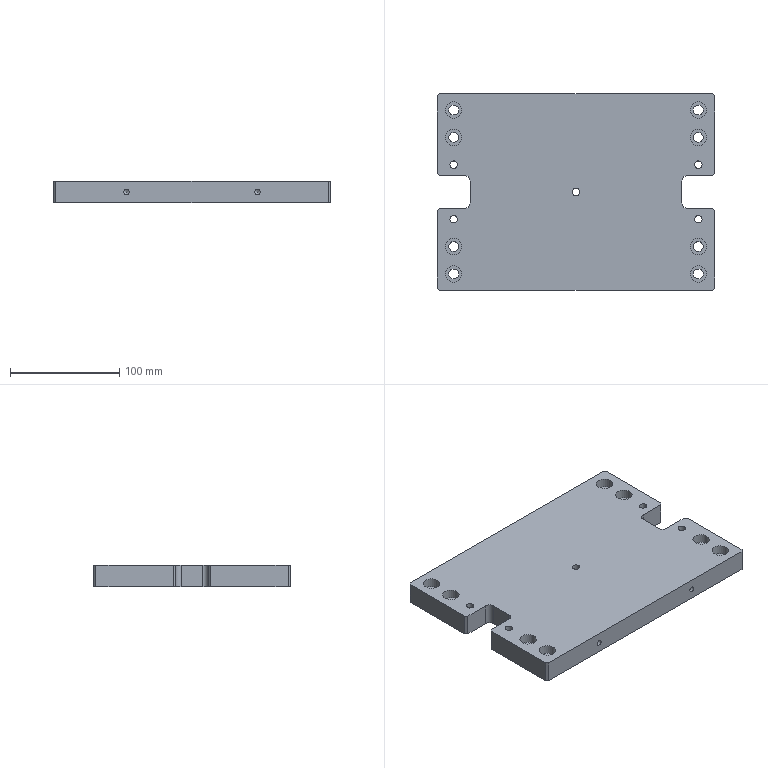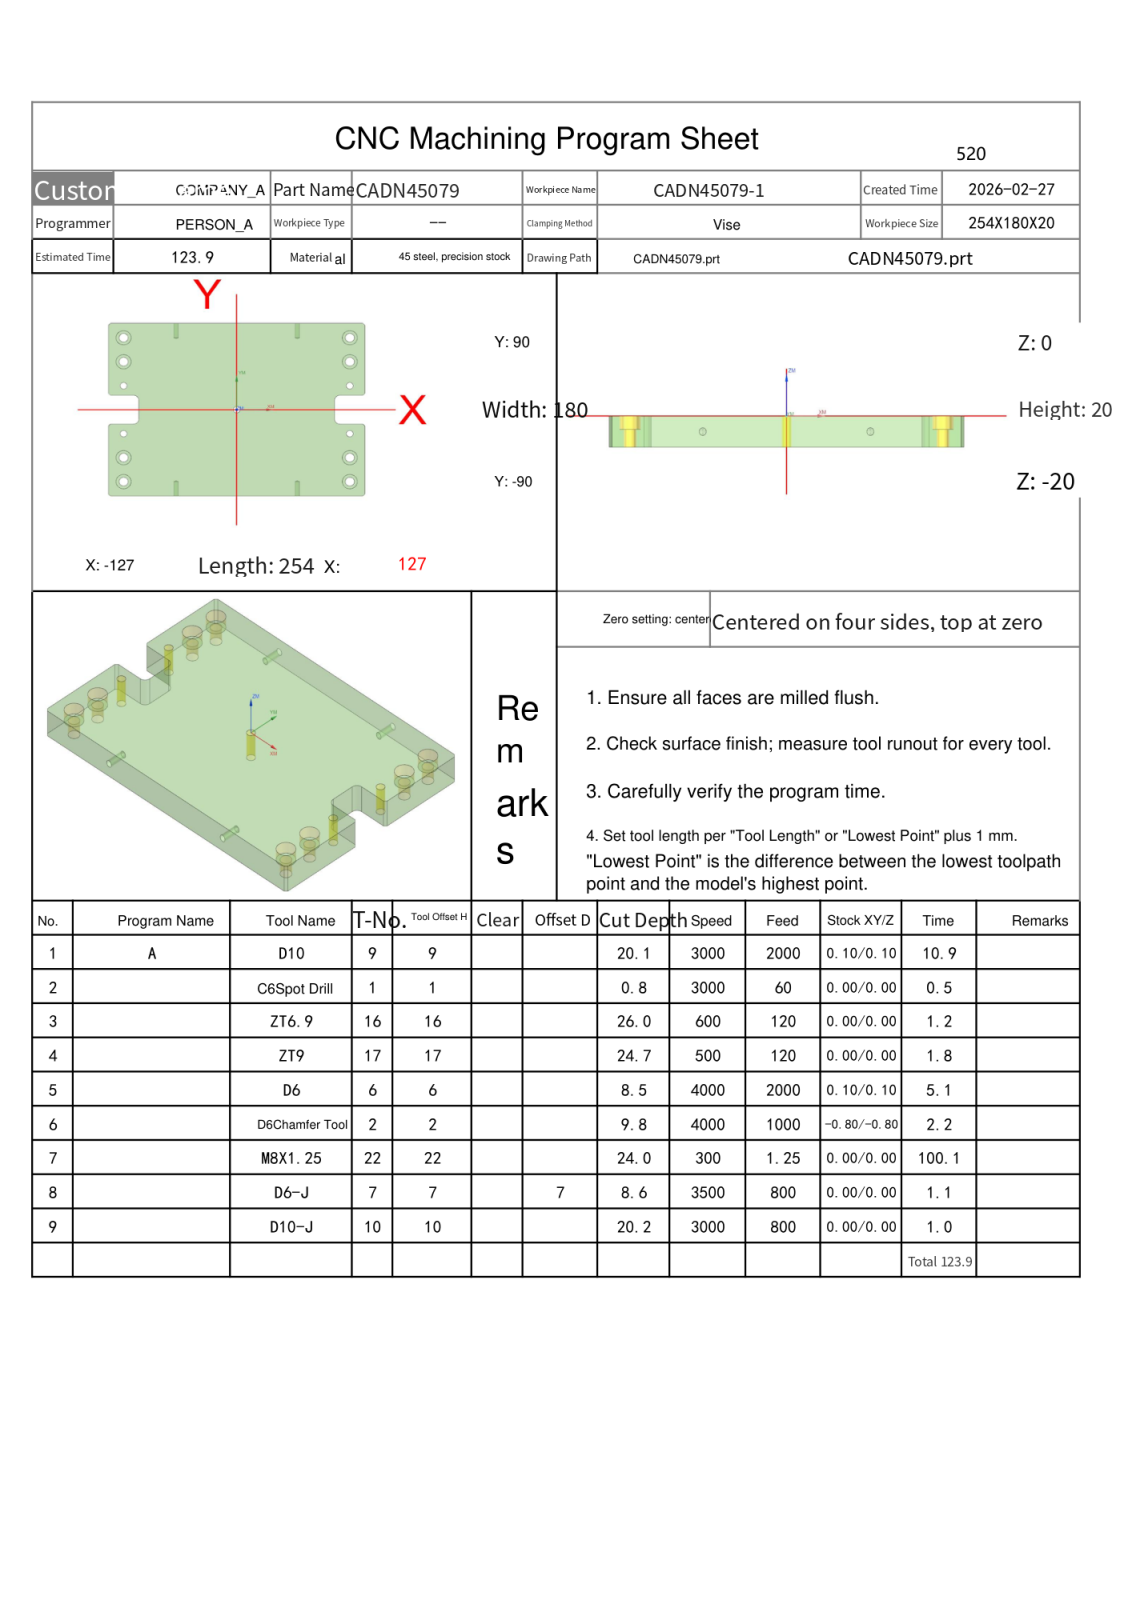NC program | NX | posted by the shop | part box 254 x 180 x 20 mm
Lines 1 to 2474 of 5116, first 2093 of 2472 lines:
%
O0001
(Machine time: 221.21 MIN)
(===Total Tool:9===)
(T9=D10     D=10.  R=0.   D-  H09 Z=-20.1 )
(T1=C6Spot Drill   D=6.   R=0.   D-  H01 Z=-0.8  )
(T16=ZT6.9  D=6.9  DR_a=120 D-  H16 Z=-26.  )
(T17=ZT9    D=9.   DR_a=118 D-  H17 Z=-24.7 )
(T6=D6      D=6.   R=0.   D-  H06 Z=-8.5  )
(T2=D6Chamfer Tool   D=6.   R=0.   D-  H02 Z=-9.8  )
(T22=M8X1.25 D=6.8  DR_a=180 D-  H22 Z=-24.  )
(T7=D6-J    D=6.   R=0.   D7  H07 Z=-8.6  )
(T10=D10-J  D=10.  R=0.   D-  H10 Z=-20.2 )
G80 G90 G17 G49 G40
G91 G28 Z0
M01
N1 T09 M06
(D10  D=10. R=0. H=09 ce=0.10 di=0.10)
G00 G90 G54 X-122.242 Y-99.97 M03 S3000
G43 H09 Z30.
M08
Z-.5
G01 X-128.606 Y-93.606 F2000.
X-130.606 Y-91.606
X-136.97 Y-85.242
G00 Z-1.
G01 X-130.606 Y-91.606
X-128.606 Y-93.606
X-122.242 Y-99.97
G00 Z-1.5
G01 X-128.606 Y-93.606
X-130.606 Y-91.606
X-136.97 Y-85.242
G00 Z-2.
G01 X-130.606 Y-91.606
X-128.606 Y-93.606
X-122.242 Y-99.97
G00 Z-2.5
G01 X-128.606 Y-93.606
X-130.606 Y-91.606
X-136.97 Y-85.242
G00 Z-3.
G01 X-130.606 Y-91.606
X-128.606 Y-93.606
X-122.242 Y-99.97
G00 Z-3.5
G01 X-128.606 Y-93.606
X-130.606 Y-91.606
X-136.97 Y-85.242
G00 Z-4.
G01 X-130.606 Y-91.606
X-128.606 Y-93.606
X-122.242 Y-99.97
G00 Z-4.5
G01 X-128.606 Y-93.606
X-130.606 Y-91.606
X-136.97 Y-85.242
G00 Z-5.
G01 X-130.606 Y-91.606
X-128.606 Y-93.606
X-122.242 Y-99.97
G00 Z-5.5
G01 X-128.606 Y-93.606
X-130.606 Y-91.606
X-136.97 Y-85.242
G00 Z-6.
G01 X-130.606 Y-91.606
X-128.606 Y-93.606
X-122.242 Y-99.97
G00 Z-6.5
G01 X-128.606 Y-93.606
X-130.606 Y-91.606
X-136.97 Y-85.242
G00 Z-7.
G01 X-130.606 Y-91.606
X-128.606 Y-93.606
X-122.242 Y-99.97
G00 Z-7.5
G01 X-128.606 Y-93.606
X-130.606 Y-91.606
X-136.97 Y-85.242
G00 Z-8.
G01 X-130.606 Y-91.606
X-128.606 Y-93.606
X-122.242 Y-99.97
G00 Z-8.5
G01 X-128.606 Y-93.606
X-130.606 Y-91.606
X-136.97 Y-85.242
G00 Z-9.
G01 X-130.606 Y-91.606
X-128.606 Y-93.606
X-122.242 Y-99.97
G00 Z-9.5
G01 X-128.606 Y-93.606
X-130.606 Y-91.606
X-136.97 Y-85.242
G00 Z-10.
G01 X-130.606 Y-91.606
X-128.606 Y-93.606
X-122.242 Y-99.97
G00 Z-10.5
G01 X-128.606 Y-93.606
X-130.606 Y-91.606
X-136.97 Y-85.242
G00 Z-10.9
G01 X-130.606 Y-91.606
X-128.606 Y-93.606
X-122.242 Y-99.97
G00 Z30.
X-136.97 Y85.242
Z-.5
G01 X-130.606 Y91.606
X-128.606 Y93.606
X-122.242 Y99.97
G00 Z-1.
G01 X-128.606 Y93.606
X-130.606 Y91.606
X-136.97 Y85.242
G00 Z-1.5
G01 X-130.606 Y91.606
X-128.606 Y93.606
X-122.242 Y99.97
G00 Z-2.
G01 X-128.606 Y93.606
X-130.606 Y91.606
X-136.97 Y85.242
G00 Z-2.5
G01 X-130.606 Y91.606
X-128.606 Y93.606
X-122.242 Y99.97
G00 Z-3.
G01 X-128.606 Y93.606
X-130.606 Y91.606
X-136.97 Y85.242
G00 Z-3.5
G01 X-130.606 Y91.606
X-128.606 Y93.606
X-122.242 Y99.97
G00 Z-4.
G01 X-128.606 Y93.606
X-130.606 Y91.606
X-136.97 Y85.242
G00 Z-4.5
G01 X-130.606 Y91.606
X-128.606 Y93.606
X-122.242 Y99.97
G00 Z-5.
G01 X-128.606 Y93.606
X-130.606 Y91.606
X-136.97 Y85.242
G00 Z-5.5
G01 X-130.606 Y91.606
X-128.606 Y93.606
X-122.242 Y99.97
G00 Z-6.
G01 X-128.606 Y93.606
X-130.606 Y91.606
X-136.97 Y85.242
G00 Z-6.5
G01 X-130.606 Y91.606
X-128.606 Y93.606
X-122.242 Y99.97
G00 Z-7.
G01 X-128.606 Y93.606
X-130.606 Y91.606
X-136.97 Y85.242
G00 Z-7.5
G01 X-130.606 Y91.606
X-128.606 Y93.606
X-122.242 Y99.97
G00 Z-8.
G01 X-128.606 Y93.606
X-130.606 Y91.606
X-136.97 Y85.242
G00 Z-8.5
G01 X-130.606 Y91.606
X-128.606 Y93.606
X-122.242 Y99.97
G00 Z-9.
G01 X-128.606 Y93.606
X-130.606 Y91.606
X-136.97 Y85.242
G00 Z-9.5
G01 X-130.606 Y91.606
X-128.606 Y93.606
X-122.242 Y99.97
G00 Z-10.
G01 X-128.606 Y93.606
X-130.606 Y91.606
X-136.97 Y85.242
G00 Z-10.5
G01 X-130.606 Y91.606
X-128.606 Y93.606
X-122.242 Y99.97
G00 Z-10.9
G01 X-128.606 Y93.606
X-130.606 Y91.606
X-136.97 Y85.242
G00 Z30.
X122.242 Y99.97
Z-.5
G01 X128.606 Y93.606
X130.606 Y91.606
X136.97 Y85.242
G00 Z-1.
G01 X130.606 Y91.606
X128.606 Y93.606
X122.242 Y99.97
G00 Z-1.5
G01 X128.606 Y93.606
X130.606 Y91.606
X136.97 Y85.242
G00 Z-2.
G01 X130.606 Y91.606
X128.606 Y93.606
X122.242 Y99.97
G00 Z-2.5
G01 X128.606 Y93.606
X130.606 Y91.606
X136.97 Y85.242
G00 Z-3.
G01 X130.606 Y91.606
X128.606 Y93.606
X122.242 Y99.97
G00 Z-3.5
G01 X128.606 Y93.606
X130.606 Y91.606
X136.97 Y85.242
G00 Z-4.
G01 X130.606 Y91.606
X128.606 Y93.606
X122.242 Y99.97
G00 Z-4.5
G01 X128.606 Y93.606
X130.606 Y91.606
X136.97 Y85.242
G00 Z-5.
G01 X130.606 Y91.606
X128.606 Y93.606
X122.242 Y99.97
G00 Z-5.5
G01 X128.606 Y93.606
X130.606 Y91.606
X136.97 Y85.242
G00 Z-6.
G01 X130.606 Y91.606
X128.606 Y93.606
X122.242 Y99.97
G00 Z-6.5
G01 X128.606 Y93.606
X130.606 Y91.606
X136.97 Y85.242
G00 Z-7.
G01 X130.606 Y91.606
X128.606 Y93.606
X122.242 Y99.97
G00 Z-7.5
G01 X128.606 Y93.606
X130.606 Y91.606
X136.97 Y85.242
G00 Z-8.
G01 X130.606 Y91.606
X128.606 Y93.606
X122.242 Y99.97
G00 Z-8.5
G01 X128.606 Y93.606
X130.606 Y91.606
X136.97 Y85.242
G00 Z-9.
G01 X130.606 Y91.606
X128.606 Y93.606
X122.242 Y99.97
G00 Z-9.5
G01 X128.606 Y93.606
X130.606 Y91.606
X136.97 Y85.242
G00 Z-10.
G01 X130.606 Y91.606
X128.606 Y93.606
X122.242 Y99.97
G00 Z-10.5
G01 X128.606 Y93.606
X130.606 Y91.606
X136.97 Y85.242
G00 Z-10.9
G01 X130.606 Y91.606
X128.606 Y93.606
X122.242 Y99.97
G00 Z30.
X136.97 Y-85.242
Z-.5
G01 X130.606 Y-91.606
X128.606 Y-93.606
X122.242 Y-99.97
G00 Z-1.
G01 X128.606 Y-93.606
X130.606 Y-91.606
X136.97 Y-85.242
G00 Z-1.5
G01 X130.606 Y-91.606
X128.606 Y-93.606
X122.242 Y-99.97
G00 Z-2.
G01 X128.606 Y-93.606
X130.606 Y-91.606
X136.97 Y-85.242
G00 Z-2.5
G01 X130.606 Y-91.606
X128.606 Y-93.606
X122.242 Y-99.97
G00 Z-3.
G01 X128.606 Y-93.606
X130.606 Y-91.606
X136.97 Y-85.242
G00 Z-3.5
G01 X130.606 Y-91.606
X128.606 Y-93.606
X122.242 Y-99.97
G00 Z-4.
G01 X128.606 Y-93.606
X130.606 Y-91.606
X136.97 Y-85.242
G00 Z-4.5
G01 X130.606 Y-91.606
X128.606 Y-93.606
X122.242 Y-99.97
G00 Z-5.
G01 X128.606 Y-93.606
X130.606 Y-91.606
X136.97 Y-85.242
G00 Z-5.5
G01 X130.606 Y-91.606
X128.606 Y-93.606
X122.242 Y-99.97
G00 Z-6.
G01 X128.606 Y-93.606
X130.606 Y-91.606
X136.97 Y-85.242
G00 Z-6.5
G01 X130.606 Y-91.606
X128.606 Y-93.606
X122.242 Y-99.97
G00 Z-7.
G01 X128.606 Y-93.606
X130.606 Y-91.606
X136.97 Y-85.242
G00 Z-7.5
G01 X130.606 Y-91.606
X128.606 Y-93.606
X122.242 Y-99.97
G00 Z-8.
G01 X128.606 Y-93.606
X130.606 Y-91.606
X136.97 Y-85.242
G00 Z-8.5
G01 X130.606 Y-91.606
X128.606 Y-93.606
X122.242 Y-99.97
G00 Z-9.
G01 X128.606 Y-93.606
X130.606 Y-91.606
X136.97 Y-85.242
G00 Z-9.5
G01 X130.606 Y-91.606
X128.606 Y-93.606
X122.242 Y-99.97
G00 Z-10.
G01 X128.606 Y-93.606
X130.606 Y-91.606
X136.97 Y-85.242
G00 Z-10.5
G01 X130.606 Y-91.606
X128.606 Y-93.606
X122.242 Y-99.97
G00 Z-10.9
G01 X128.606 Y-93.606
X130.606 Y-91.606
X136.97 Y-85.242
G00 Z30.
G00 G90 X-136.97 Y-19.758 M03 S3000
Z30.
Z-.2
G01 X-130.606 Y-13.394 F2000.
X-128.606 Y-11.394
G02 X-125. Y-9.9 I3.606 J-3.606
G01 X-102.1
Y9.9
X-125.
G02 X-128.606 Y11.394 I0.0 J5.1
G01 X-130.606 Y13.394
X-136.97 Y19.758
G00 Z-.4
G01 X-130.606 Y13.394
X-128.606 Y11.394
G03 X-125. Y9.9 I3.606 J3.606
G01 X-102.1
Y-9.9
X-125.
G03 X-128.606 Y-11.394 I0.0 J-5.1
G01 X-130.606 Y-13.394
X-136.97 Y-19.758
G00 Z-.6
G01 X-130.606 Y-13.394
X-128.606 Y-11.394
G02 X-125. Y-9.9 I3.606 J-3.606
G01 X-102.1
Y9.9
X-125.
G02 X-128.606 Y11.394 I0.0 J5.1
G01 X-130.606 Y13.394
X-136.97 Y19.758
G00 Z-.8
G01 X-130.606 Y13.394
X-128.606 Y11.394
G03 X-125. Y9.9 I3.606 J3.606
G01 X-102.1
Y-9.9
X-125.
G03 X-128.606 Y-11.394 I0.0 J-5.1
G01 X-130.606 Y-13.394
X-136.97 Y-19.758
G00 Z-1.
G01 X-130.606 Y-13.394
X-128.606 Y-11.394
G02 X-125. Y-9.9 I3.606 J-3.606
G01 X-102.1
Y9.9
X-125.
G02 X-128.606 Y11.394 I0.0 J5.1
G01 X-130.606 Y13.394
X-136.97 Y19.758
G00 Z-1.2
G01 X-130.606 Y13.394
X-128.606 Y11.394
G03 X-125. Y9.9 I3.606 J3.606
G01 X-102.1
Y-9.9
X-125.
G03 X-128.606 Y-11.394 I0.0 J-5.1
G01 X-130.606 Y-13.394
X-136.97 Y-19.758
G00 Z-1.4
G01 X-130.606 Y-13.394
X-128.606 Y-11.394
G02 X-125. Y-9.9 I3.606 J-3.606
G01 X-102.1
Y9.9
X-125.
G02 X-128.606 Y11.394 I0.0 J5.1
G01 X-130.606 Y13.394
X-136.97 Y19.758
G00 Z-1.6
G01 X-130.606 Y13.394
X-128.606 Y11.394
G03 X-125. Y9.9 I3.606 J3.606
G01 X-102.1
Y-9.9
X-125.
G03 X-128.606 Y-11.394 I0.0 J-5.1
G01 X-130.606 Y-13.394
X-136.97 Y-19.758
G00 Z-1.8
G01 X-130.606 Y-13.394
X-128.606 Y-11.394
G02 X-125. Y-9.9 I3.606 J-3.606
G01 X-102.1
Y9.9
X-125.
G02 X-128.606 Y11.394 I0.0 J5.1
G01 X-130.606 Y13.394
X-136.97 Y19.758
G00 Z-2.
G01 X-130.606 Y13.394
X-128.606 Y11.394
G03 X-125. Y9.9 I3.606 J3.606
G01 X-102.1
Y-9.9
X-125.
G03 X-128.606 Y-11.394 I0.0 J-5.1
G01 X-130.606 Y-13.394
X-136.97 Y-19.758
G00 Z-2.2
G01 X-130.606 Y-13.394
X-128.606 Y-11.394
G02 X-125. Y-9.9 I3.606 J-3.606
G01 X-102.1
Y9.9
X-125.
G02 X-128.606 Y11.394 I0.0 J5.1
G01 X-130.606 Y13.394
X-136.97 Y19.758
G00 Z-2.4
G01 X-130.606 Y13.394
X-128.606 Y11.394
G03 X-125. Y9.9 I3.606 J3.606
G01 X-102.1
Y-9.9
X-125.
G03 X-128.606 Y-11.394 I0.0 J-5.1
G01 X-130.606 Y-13.394
X-136.97 Y-19.758
G00 Z-2.6
G01 X-130.606 Y-13.394
X-128.606 Y-11.394
G02 X-125. Y-9.9 I3.606 J-3.606
G01 X-102.1
Y9.9
X-125.
G02 X-128.606 Y11.394 I0.0 J5.1
G01 X-130.606 Y13.394
X-136.97 Y19.758
G00 Z-2.8
G01 X-130.606 Y13.394
X-128.606 Y11.394
G03 X-125. Y9.9 I3.606 J3.606
G01 X-102.1
Y-9.9
X-125.
G03 X-128.606 Y-11.394 I0.0 J-5.1
G01 X-130.606 Y-13.394
X-136.97 Y-19.758
G00 Z-3.
G01 X-130.606 Y-13.394
X-128.606 Y-11.394
G02 X-125. Y-9.9 I3.606 J-3.606
G01 X-102.1
Y9.9
X-125.
G02 X-128.606 Y11.394 I0.0 J5.1
G01 X-130.606 Y13.394
X-136.97 Y19.758
G00 Z-3.2
G01 X-130.606 Y13.394
X-128.606 Y11.394
G03 X-125. Y9.9 I3.606 J3.606
G01 X-102.1
Y-9.9
X-125.
G03 X-128.606 Y-11.394 I0.0 J-5.1
G01 X-130.606 Y-13.394
X-136.97 Y-19.758
G00 Z-3.4
G01 X-130.606 Y-13.394
X-128.606 Y-11.394
G02 X-125. Y-9.9 I3.606 J-3.606
G01 X-102.1
Y9.9
X-125.
G02 X-128.606 Y11.394 I0.0 J5.1
G01 X-130.606 Y13.394
X-136.97 Y19.758
G00 Z-3.6
G01 X-130.606 Y13.394
X-128.606 Y11.394
G03 X-125. Y9.9 I3.606 J3.606
G01 X-102.1
Y-9.9
X-125.
G03 X-128.606 Y-11.394 I0.0 J-5.1
G01 X-130.606 Y-13.394
X-136.97 Y-19.758
G00 Z-3.8
G01 X-130.606 Y-13.394
X-128.606 Y-11.394
G02 X-125. Y-9.9 I3.606 J-3.606
G01 X-102.1
Y9.9
X-125.
G02 X-128.606 Y11.394 I0.0 J5.1
G01 X-130.606 Y13.394
X-136.97 Y19.758
G00 Z-4.
G01 X-130.606 Y13.394
X-128.606 Y11.394
G03 X-125. Y9.9 I3.606 J3.606
G01 X-102.1
Y-9.9
X-125.
G03 X-128.606 Y-11.394 I0.0 J-5.1
G01 X-130.606 Y-13.394
X-136.97 Y-19.758
G00 Z-4.2
G01 X-130.606 Y-13.394
X-128.606 Y-11.394
G02 X-125. Y-9.9 I3.606 J-3.606
G01 X-102.1
Y9.9
X-125.
G02 X-128.606 Y11.394 I0.0 J5.1
G01 X-130.606 Y13.394
X-136.97 Y19.758
G00 Z-4.4
G01 X-130.606 Y13.394
X-128.606 Y11.394
G03 X-125. Y9.9 I3.606 J3.606
G01 X-102.1
Y-9.9
X-125.
G03 X-128.606 Y-11.394 I0.0 J-5.1
G01 X-130.606 Y-13.394
X-136.97 Y-19.758
G00 Z-4.6
G01 X-130.606 Y-13.394
X-128.606 Y-11.394
G02 X-125. Y-9.9 I3.606 J-3.606
G01 X-102.1
Y9.9
X-125.
G02 X-128.606 Y11.394 I0.0 J5.1
G01 X-130.606 Y13.394
X-136.97 Y19.758
G00 Z-4.8
G01 X-130.606 Y13.394
X-128.606 Y11.394
G03 X-125. Y9.9 I3.606 J3.606
G01 X-102.1
Y-9.9
X-125.
G03 X-128.606 Y-11.394 I0.0 J-5.1
G01 X-130.606 Y-13.394
X-136.97 Y-19.758
G00 Z-5.
G01 X-130.606 Y-13.394
X-128.606 Y-11.394
G02 X-125. Y-9.9 I3.606 J-3.606
G01 X-102.1
Y9.9
X-125.
G02 X-128.606 Y11.394 I0.0 J5.1
G01 X-130.606 Y13.394
X-136.97 Y19.758
G00 Z-5.2
G01 X-130.606 Y13.394
X-128.606 Y11.394
G03 X-125. Y9.9 I3.606 J3.606
G01 X-102.1
Y-9.9
X-125.
G03 X-128.606 Y-11.394 I0.0 J-5.1
G01 X-130.606 Y-13.394
X-136.97 Y-19.758
G00 Z-5.4
G01 X-130.606 Y-13.394
X-128.606 Y-11.394
G02 X-125. Y-9.9 I3.606 J-3.606
G01 X-102.1
Y9.9
X-125.
G02 X-128.606 Y11.394 I0.0 J5.1
G01 X-130.606 Y13.394
X-136.97 Y19.758
G00 Z-5.6
G01 X-130.606 Y13.394
X-128.606 Y11.394
G03 X-125. Y9.9 I3.606 J3.606
G01 X-102.1
Y-9.9
X-125.
G03 X-128.606 Y-11.394 I0.0 J-5.1
G01 X-130.606 Y-13.394
X-136.97 Y-19.758
G00 Z-5.8
G01 X-130.606 Y-13.394
X-128.606 Y-11.394
G02 X-125. Y-9.9 I3.606 J-3.606
G01 X-102.1
Y9.9
X-125.
G02 X-128.606 Y11.394 I0.0 J5.1
G01 X-130.606 Y13.394
X-136.97 Y19.758
G00 Z-6.
G01 X-130.606 Y13.394
X-128.606 Y11.394
G03 X-125. Y9.9 I3.606 J3.606
G01 X-102.1
Y-9.9
X-125.
G03 X-128.606 Y-11.394 I0.0 J-5.1
G01 X-130.606 Y-13.394
X-136.97 Y-19.758
G00 Z-6.2
G01 X-130.606 Y-13.394
X-128.606 Y-11.394
G02 X-125. Y-9.9 I3.606 J-3.606
G01 X-102.1
Y9.9
X-125.
G02 X-128.606 Y11.394 I0.0 J5.1
G01 X-130.606 Y13.394
X-136.97 Y19.758
G00 Z-6.4
G01 X-130.606 Y13.394
X-128.606 Y11.394
G03 X-125. Y9.9 I3.606 J3.606
G01 X-102.1
Y-9.9
X-125.
G03 X-128.606 Y-11.394 I0.0 J-5.1
G01 X-130.606 Y-13.394
X-136.97 Y-19.758
G00 Z-6.6
G01 X-130.606 Y-13.394
X-128.606 Y-11.394
G02 X-125. Y-9.9 I3.606 J-3.606
G01 X-102.1
Y9.9
X-125.
G02 X-128.606 Y11.394 I0.0 J5.1
G01 X-130.606 Y13.394
X-136.97 Y19.758
G00 Z-6.8
G01 X-130.606 Y13.394
X-128.606 Y11.394
G03 X-125. Y9.9 I3.606 J3.606
G01 X-102.1
Y-9.9
X-125.
G03 X-128.606 Y-11.394 I0.0 J-5.1
G01 X-130.606 Y-13.394
X-136.97 Y-19.758
G00 Z-7.
G01 X-130.606 Y-13.394
X-128.606 Y-11.394
G02 X-125. Y-9.9 I3.606 J-3.606
G01 X-102.1
Y9.9
X-125.
G02 X-128.606 Y11.394 I0.0 J5.1
G01 X-130.606 Y13.394
X-136.97 Y19.758
G00 Z-7.2
G01 X-130.606 Y13.394
X-128.606 Y11.394
G03 X-125. Y9.9 I3.606 J3.606
G01 X-102.1
Y-9.9
X-125.
G03 X-128.606 Y-11.394 I0.0 J-5.1
G01 X-130.606 Y-13.394
X-136.97 Y-19.758
G00 Z-7.4
G01 X-130.606 Y-13.394
X-128.606 Y-11.394
G02 X-125. Y-9.9 I3.606 J-3.606
G01 X-102.1
Y9.9
X-125.
G02 X-128.606 Y11.394 I0.0 J5.1
G01 X-130.606 Y13.394
X-136.97 Y19.758
G00 Z-7.6
G01 X-130.606 Y13.394
X-128.606 Y11.394
G03 X-125. Y9.9 I3.606 J3.606
G01 X-102.1
Y-9.9
X-125.
G03 X-128.606 Y-11.394 I0.0 J-5.1
G01 X-130.606 Y-13.394
X-136.97 Y-19.758
G00 Z-7.8
G01 X-130.606 Y-13.394
X-128.606 Y-11.394
G02 X-125. Y-9.9 I3.606 J-3.606
G01 X-102.1
Y9.9
X-125.
G02 X-128.606 Y11.394 I0.0 J5.1
G01 X-130.606 Y13.394
X-136.97 Y19.758
G00 Z-8.
G01 X-130.606 Y13.394
X-128.606 Y11.394
G03 X-125. Y9.9 I3.606 J3.606
G01 X-102.1
Y-9.9
X-125.
G03 X-128.606 Y-11.394 I0.0 J-5.1
G01 X-130.606 Y-13.394
X-136.97 Y-19.758
G00 Z-8.2
G01 X-130.606 Y-13.394
X-128.606 Y-11.394
G02 X-125. Y-9.9 I3.606 J-3.606
G01 X-102.1
Y9.9
X-125.
G02 X-128.606 Y11.394 I0.0 J5.1
G01 X-130.606 Y13.394
X-136.97 Y19.758
G00 Z-8.4
G01 X-130.606 Y13.394
X-128.606 Y11.394
G03 X-125. Y9.9 I3.606 J3.606
G01 X-102.1
Y-9.9
X-125.
G03 X-128.606 Y-11.394 I0.0 J-5.1
G01 X-130.606 Y-13.394
X-136.97 Y-19.758
G00 Z-8.6
G01 X-130.606 Y-13.394
X-128.606 Y-11.394
G02 X-125. Y-9.9 I3.606 J-3.606
G01 X-102.1
Y9.9
X-125.
G02 X-128.606 Y11.394 I0.0 J5.1
G01 X-130.606 Y13.394
X-136.97 Y19.758
G00 Z-8.8
G01 X-130.606 Y13.394
X-128.606 Y11.394
G03 X-125. Y9.9 I3.606 J3.606
G01 X-102.1
Y-9.9
X-125.
G03 X-128.606 Y-11.394 I0.0 J-5.1
G01 X-130.606 Y-13.394
X-136.97 Y-19.758
G00 Z-9.
G01 X-130.606 Y-13.394
X-128.606 Y-11.394
G02 X-125. Y-9.9 I3.606 J-3.606
G01 X-102.1
Y9.9
X-125.
G02 X-128.606 Y11.394 I0.0 J5.1
G01 X-130.606 Y13.394
X-136.97 Y19.758
G00 Z-9.2
G01 X-130.606 Y13.394
X-128.606 Y11.394
G03 X-125. Y9.9 I3.606 J3.606
G01 X-102.1
Y-9.9
X-125.
G03 X-128.606 Y-11.394 I0.0 J-5.1
G01 X-130.606 Y-13.394
X-136.97 Y-19.758
G00 Z-9.4
G01 X-130.606 Y-13.394
X-128.606 Y-11.394
G02 X-125. Y-9.9 I3.606 J-3.606
G01 X-102.1
Y9.9
X-125.
G02 X-128.606 Y11.394 I0.0 J5.1
G01 X-130.606 Y13.394
X-136.97 Y19.758
G00 Z-9.6
G01 X-130.606 Y13.394
X-128.606 Y11.394
G03 X-125. Y9.9 I3.606 J3.606
G01 X-102.1
Y-9.9
X-125.
G03 X-128.606 Y-11.394 I0.0 J-5.1
G01 X-130.606 Y-13.394
X-136.97 Y-19.758
G00 Z-9.8
G01 X-130.606 Y-13.394
X-128.606 Y-11.394
G02 X-125. Y-9.9 I3.606 J-3.606
G01 X-102.1
Y9.9
X-125.
G02 X-128.606 Y11.394 I0.0 J5.1
G01 X-130.606 Y13.394
X-136.97 Y19.758
G00 Z-10.
G01 X-130.606 Y13.394
X-128.606 Y11.394
G03 X-125. Y9.9 I3.606 J3.606
G01 X-102.1
Y-9.9
X-125.
G03 X-128.606 Y-11.394 I0.0 J-5.1
G01 X-130.606 Y-13.394
X-136.97 Y-19.758
G00 Z-10.2
G01 X-130.606 Y-13.394
X-128.606 Y-11.394
G02 X-125. Y-9.9 I3.606 J-3.606
G01 X-102.1
Y9.9
X-125.
G02 X-128.606 Y11.394 I0.0 J5.1
G01 X-130.606 Y13.394
X-136.97 Y19.758
G00 Z-10.4
G01 X-130.606 Y13.394
X-128.606 Y11.394
G03 X-125. Y9.9 I3.606 J3.606
G01 X-102.1
Y-9.9
X-125.
G03 X-128.606 Y-11.394 I0.0 J-5.1
G01 X-130.606 Y-13.394
X-136.97 Y-19.758
G00 Z-10.6
G01 X-130.606 Y-13.394
X-128.606 Y-11.394
G02 X-125. Y-9.9 I3.606 J-3.606
G01 X-102.1
Y9.9
X-125.
G02 X-128.606 Y11.394 I0.0 J5.1
G01 X-130.606 Y13.394
X-136.97 Y19.758
G00 Z-10.8
G01 X-130.606 Y13.394
X-128.606 Y11.394
G03 X-125. Y9.9 I3.606 J3.606
G01 X-102.1
Y-9.9
X-125.
G03 X-128.606 Y-11.394 I0.0 J-5.1
G01 X-130.606 Y-13.394
X-136.97 Y-19.758
G00 Z-11.
G01 X-130.606 Y-13.394
X-128.606 Y-11.394
G02 X-125. Y-9.9 I3.606 J-3.606
G01 X-102.1
Y9.9
X-125.
G02 X-128.606 Y11.394 I0.0 J5.1
G01 X-130.606 Y13.394
X-136.97 Y19.758
G00 Z-11.2
G01 X-130.606 Y13.394
X-128.606 Y11.394
G03 X-125. Y9.9 I3.606 J3.606
G01 X-102.1
Y-9.9
X-125.
G03 X-128.606 Y-11.394 I0.0 J-5.1
G01 X-130.606 Y-13.394
X-136.97 Y-19.758
G00 Z-11.4
G01 X-130.606 Y-13.394
X-128.606 Y-11.394
G02 X-125. Y-9.9 I3.606 J-3.606
G01 X-102.1
Y9.9
X-125.
G02 X-128.606 Y11.394 I0.0 J5.1
G01 X-130.606 Y13.394
X-136.97 Y19.758
G00 Z-11.6
G01 X-130.606 Y13.394
X-128.606 Y11.394
G03 X-125. Y9.9 I3.606 J3.606
G01 X-102.1
Y-9.9
X-125.
G03 X-128.606 Y-11.394 I0.0 J-5.1
G01 X-130.606 Y-13.394
X-136.97 Y-19.758
G00 Z-11.8
G01 X-130.606 Y-13.394
X-128.606 Y-11.394
G02 X-125. Y-9.9 I3.606 J-3.606
G01 X-102.1
Y9.9
X-125.
G02 X-128.606 Y11.394 I0.0 J5.1
G01 X-130.606 Y13.394
X-136.97 Y19.758
G00 Z-12.
G01 X-130.606 Y13.394
X-128.606 Y11.394
G03 X-125. Y9.9 I3.606 J3.606
G01 X-102.1
Y-9.9
X-125.
G03 X-128.606 Y-11.394 I0.0 J-5.1
G01 X-130.606 Y-13.394
X-136.97 Y-19.758
G00 Z-12.2
G01 X-130.606 Y-13.394
X-128.606 Y-11.394
G02 X-125. Y-9.9 I3.606 J-3.606
G01 X-102.1
Y9.9
X-125.
G02 X-128.606 Y11.394 I0.0 J5.1
G01 X-130.606 Y13.394
X-136.97 Y19.758
G00 Z-12.4
G01 X-130.606 Y13.394
X-128.606 Y11.394
G03 X-125. Y9.9 I3.606 J3.606
G01 X-102.1
Y-9.9
X-125.
G03 X-128.606 Y-11.394 I0.0 J-5.1
G01 X-130.606 Y-13.394
X-136.97 Y-19.758
G00 Z-12.6
G01 X-130.606 Y-13.394
X-128.606 Y-11.394
G02 X-125. Y-9.9 I3.606 J-3.606
G01 X-102.1
Y9.9
X-125.
G02 X-128.606 Y11.394 I0.0 J5.1
G01 X-130.606 Y13.394
X-136.97 Y19.758
G00 Z-12.8
G01 X-130.606 Y13.394
X-128.606 Y11.394
G03 X-125. Y9.9 I3.606 J3.606
G01 X-102.1
Y-9.9
X-125.
G03 X-128.606 Y-11.394 I0.0 J-5.1
G01 X-130.606 Y-13.394
X-136.97 Y-19.758
G00 Z-13.
G01 X-130.606 Y-13.394
X-128.606 Y-11.394
G02 X-125. Y-9.9 I3.606 J-3.606
G01 X-102.1
Y9.9
X-125.
G02 X-128.606 Y11.394 I0.0 J5.1
G01 X-130.606 Y13.394
X-136.97 Y19.758
G00 Z-13.2
G01 X-130.606 Y13.394
X-128.606 Y11.394
G03 X-125. Y9.9 I3.606 J3.606
G01 X-102.1
Y-9.9
X-125.
G03 X-128.606 Y-11.394 I0.0 J-5.1
G01 X-130.606 Y-13.394
X-136.97 Y-19.758
G00 Z-13.4
G01 X-130.606 Y-13.394
X-128.606 Y-11.394
G02 X-125. Y-9.9 I3.606 J-3.606
G01 X-102.1
Y9.9
X-125.
G02 X-128.606 Y11.394 I0.0 J5.1
G01 X-130.606 Y13.394
X-136.97 Y19.758
G00 Z-13.6
G01 X-130.606 Y13.394
X-128.606 Y11.394
G03 X-125. Y9.9 I3.606 J3.606
G01 X-102.1
Y-9.9
X-125.
G03 X-128.606 Y-11.394 I0.0 J-5.1
G01 X-130.606 Y-13.394
X-136.97 Y-19.758
G00 Z-13.8
G01 X-130.606 Y-13.394
X-128.606 Y-11.394
G02 X-125. Y-9.9 I3.606 J-3.606
G01 X-102.1
Y9.9
X-125.
G02 X-128.606 Y11.394 I0.0 J5.1
G01 X-130.606 Y13.394
X-136.97 Y19.758
G00 Z-14.
G01 X-130.606 Y13.394
X-128.606 Y11.394
G03 X-125. Y9.9 I3.606 J3.606
G01 X-102.1
Y-9.9
X-125.
G03 X-128.606 Y-11.394 I0.0 J-5.1
G01 X-130.606 Y-13.394
X-136.97 Y-19.758
G00 Z-14.2
G01 X-130.606 Y-13.394
X-128.606 Y-11.394
G02 X-125. Y-9.9 I3.606 J-3.606
G01 X-102.1
Y9.9
X-125.
G02 X-128.606 Y11.394 I0.0 J5.1
G01 X-130.606 Y13.394
X-136.97 Y19.758
G00 Z-14.4
G01 X-130.606 Y13.394
X-128.606 Y11.394
G03 X-125. Y9.9 I3.606 J3.606
G01 X-102.1
Y-9.9
X-125.
G03 X-128.606 Y-11.394 I0.0 J-5.1
G01 X-130.606 Y-13.394
X-136.97 Y-19.758
G00 Z-14.6
G01 X-130.606 Y-13.394
X-128.606 Y-11.394
G02 X-125. Y-9.9 I3.606 J-3.606
G01 X-102.1
Y9.9
X-125.
G02 X-128.606 Y11.394 I0.0 J5.1
G01 X-130.606 Y13.394
X-136.97 Y19.758
G00 Z-14.8
G01 X-130.606 Y13.394
X-128.606 Y11.394
G03 X-125. Y9.9 I3.606 J3.606
G01 X-102.1
Y-9.9
X-125.
G03 X-128.606 Y-11.394 I0.0 J-5.1
G01 X-130.606 Y-13.394
X-136.97 Y-19.758
G00 Z-15.
G01 X-130.606 Y-13.394
X-128.606 Y-11.394
G02 X-125. Y-9.9 I3.606 J-3.606
G01 X-102.1
Y9.9
X-125.
G02 X-128.606 Y11.394 I0.0 J5.1
G01 X-130.606 Y13.394
X-136.97 Y19.758
G00 Z-15.2
G01 X-130.606 Y13.394
X-128.606 Y11.394
G03 X-125. Y9.9 I3.606 J3.606
G01 X-102.1
Y-9.9
X-125.
G03 X-128.606 Y-11.394 I0.0 J-5.1
G01 X-130.606 Y-13.394
X-136.97 Y-19.758
G00 Z-15.4
G01 X-130.606 Y-13.394
X-128.606 Y-11.394
G02 X-125. Y-9.9 I3.606 J-3.606
G01 X-102.1
Y9.9
X-125.
G02 X-128.606 Y11.394 I0.0 J5.1
G01 X-130.606 Y13.394
X-136.97 Y19.758
G00 Z-15.6
G01 X-130.606 Y13.394
X-128.606 Y11.394
G03 X-125. Y9.9 I3.606 J3.606
G01 X-102.1
Y-9.9
X-125.
G03 X-128.606 Y-11.394 I0.0 J-5.1
G01 X-130.606 Y-13.394
X-136.97 Y-19.758
G00 Z-15.8
G01 X-130.606 Y-13.394
X-128.606 Y-11.394
G02 X-125. Y-9.9 I3.606 J-3.606
G01 X-102.1
Y9.9
X-125.
G02 X-128.606 Y11.394 I0.0 J5.1
G01 X-130.606 Y13.394
X-136.97 Y19.758
G00 Z-16.
G01 X-130.606 Y13.394
X-128.606 Y11.394
G03 X-125. Y9.9 I3.606 J3.606
G01 X-102.1
Y-9.9
X-125.
G03 X-128.606 Y-11.394 I0.0 J-5.1
G01 X-130.606 Y-13.394
X-136.97 Y-19.758
G00 Z-16.2
G01 X-130.606 Y-13.394
X-128.606 Y-11.394
G02 X-125. Y-9.9 I3.606 J-3.606
G01 X-102.1
Y9.9
X-125.
G02 X-128.606 Y11.394 I0.0 J5.1
G01 X-130.606 Y13.394
X-136.97 Y19.758
G00 Z-16.4
G01 X-130.606 Y13.394
X-128.606 Y11.394
G03 X-125. Y9.9 I3.606 J3.606
G01 X-102.1
Y-9.9
X-125.
G03 X-128.606 Y-11.394 I0.0 J-5.1
G01 X-130.606 Y-13.394
X-136.97 Y-19.758
G00 Z-16.6
G01 X-130.606 Y-13.394
X-128.606 Y-11.394
G02 X-125. Y-9.9 I3.606 J-3.606
G01 X-102.1
Y9.9
X-125.
G02 X-128.606 Y11.394 I0.0 J5.1
G01 X-130.606 Y13.394
X-136.97 Y19.758
G00 Z-16.8
G01 X-130.606 Y13.394
X-128.606 Y11.394
G03 X-125. Y9.9 I3.606 J3.606
G01 X-102.1
Y-9.9
X-125.
G03 X-128.606 Y-11.394 I0.0 J-5.1
G01 X-130.606 Y-13.394
X-136.97 Y-19.758
G00 Z-17.
G01 X-130.606 Y-13.394
X-128.606 Y-11.394
G02 X-125. Y-9.9 I3.606 J-3.606
G01 X-102.1
Y9.9
X-125.
G02 X-128.606 Y11.394 I0.0 J5.1
G01 X-130.606 Y13.394
X-136.97 Y19.758
G00 Z-17.2
G01 X-130.606 Y13.394
X-128.606 Y11.394
G03 X-125. Y9.9 I3.606 J3.606
G01 X-102.1
Y-9.9
X-125.
G03 X-128.606 Y-11.394 I0.0 J-5.1
G01 X-130.606 Y-13.394
X-136.97 Y-19.758
G00 Z-17.4
G01 X-130.606 Y-13.394
X-128.606 Y-11.394
G02 X-125. Y-9.9 I3.606 J-3.606
G01 X-102.1
Y9.9
X-125.
G02 X-128.606 Y11.394 I0.0 J5.1
G01 X-130.606 Y13.394
X-136.97 Y19.758
G00 Z-17.6
G01 X-130.606 Y13.394
X-128.606 Y11.394
G03 X-125. Y9.9 I3.606 J3.606
G01 X-102.1
Y-9.9
X-125.
G03 X-128.606 Y-11.394 I0.0 J-5.1
G01 X-130.606 Y-13.394
X-136.97 Y-19.758
G00 Z-17.8
G01 X-130.606 Y-13.394
X-128.606 Y-11.394
G02 X-125. Y-9.9 I3.606 J-3.606
G01 X-102.1
Y9.9
X-125.
G02 X-128.606 Y11.394 I0.0 J5.1
G01 X-130.606 Y13.394
X-136.97 Y19.758
G00 Z-18.
G01 X-130.606 Y13.394
X-128.606 Y11.394
G03 X-125. Y9.9 I3.606 J3.606
G01 X-102.1
Y-9.9
X-125.
G03 X-128.606 Y-11.394 I0.0 J-5.1
G01 X-130.606 Y-13.394
X-136.97 Y-19.758
G00 Z-18.2
G01 X-130.606 Y-13.394
X-128.606 Y-11.394
G02 X-125. Y-9.9 I3.606 J-3.606
G01 X-102.1
Y9.9
X-125.
G02 X-128.606 Y11.394 I0.0 J5.1
G01 X-130.606 Y13.394
X-136.97 Y19.758
G00 Z-18.4
G01 X-130.606 Y13.394
X-128.606 Y11.394
G03 X-125. Y9.9 I3.606 J3.606
G01 X-102.1
Y-9.9
X-125.
G03 X-128.606 Y-11.394 I0.0 J-5.1
G01 X-130.606 Y-13.394
X-136.97 Y-19.758
G00 Z-18.6
G01 X-130.606 Y-13.394
X-128.606 Y-11.394
G02 X-125. Y-9.9 I3.606 J-3.606
G01 X-102.1
Y9.9
X-125.
G02 X-128.606 Y11.394 I0.0 J5.1
G01 X-130.606 Y13.394
X-136.97 Y19.758
G00 Z-18.8
G01 X-130.606 Y13.394
X-128.606 Y11.394
G03 X-125. Y9.9 I3.606 J3.606
G01 X-102.1
Y-9.9
X-125.
G03 X-128.606 Y-11.394 I0.0 J-5.1
G01 X-130.606 Y-13.394
X-136.97 Y-19.758
G00 Z-19.
G01 X-130.606 Y-13.394
X-128.606 Y-11.394
G02 X-125. Y-9.9 I3.606 J-3.606
G01 X-102.1
Y9.9
X-125.
G02 X-128.606 Y11.394 I0.0 J5.1
G01 X-130.606 Y13.394
X-136.97 Y19.758
G00 Z-19.2
G01 X-130.606 Y13.394
X-128.606 Y11.394
G03 X-125. Y9.9 I3.606 J3.606
G01 X-102.1
Y-9.9
X-125.
G03 X-128.606 Y-11.394 I0.0 J-5.1
G01 X-130.606 Y-13.394
X-136.97 Y-19.758
G00 Z-19.4
G01 X-130.606 Y-13.394
X-128.606 Y-11.394
G02 X-125. Y-9.9 I3.606 J-3.606
G01 X-102.1
Y9.9
X-125.
G02 X-128.606 Y11.394 I0.0 J5.1
G01 X-130.606 Y13.394
X-136.97 Y19.758
G00 Z-19.6
G01 X-130.606 Y13.394
X-128.606 Y11.394
G03 X-125. Y9.9 I3.606 J3.606
G01 X-102.1
Y-9.9
X-125.
G03 X-128.606 Y-11.394 I0.0 J-5.1
G01 X-130.606 Y-13.394
X-136.97 Y-19.758
G00 Z-19.8
G01 X-130.606 Y-13.394
X-128.606 Y-11.394
G02 X-125. Y-9.9 I3.606 J-3.606
G01 X-102.1
Y9.9
X-125.
G02 X-128.606 Y11.394 I0.0 J5.1
G01 X-130.606 Y13.394
X-136.97 Y19.758
G00 Z-20.
G01 X-130.606 Y13.394
X-128.606 Y11.394
G03 X-125. Y9.9 I3.606 J3.606
G01 X-102.1
Y-9.9
X-125.
G03 X-128.606 Y-11.394 I0.0 J-5.1
G01 X-130.606 Y-13.394
X-136.97 Y-19.758
G00 Z-20.1
G01 X-130.606 Y-13.394
X-128.606 Y-11.394
G02 X-125. Y-9.9 I3.606 J-3.606
G01 X-102.1
Y9.9
X-125.
G02 X-128.606 Y11.394 I0.0 J5.1
G01 X-130.606 Y13.394
X-136.97 Y19.758
G00 Z30.
X136.97
Z-.2
G01 X130.606 Y13.394
X128.606 Y11.394
G02 X125. Y9.9 I-3.606 J3.606
G01 X102.1
Y-9.9
X125.
G02 X128.606 Y-11.394 I0.0 J-5.1
G01 X130.606 Y-13.394
X136.97 Y-19.758
G00 Z-.4
G01 X130.606 Y-13.394
X128.606 Y-11.394
G03 X125. Y-9.9 I-3.606 J-3.606
G01 X102.1
Y9.9
X125.
G03 X128.606 Y11.394 I0.0 J5.1
G01 X130.606 Y13.394
X136.97 Y19.758
G00 Z-.6
G01 X130.606 Y13.394
X128.606 Y11.394
G02 X125. Y9.9 I-3.606 J3.606
G01 X102.1
Y-9.9
X125.
G02 X128.606 Y-11.394 I0.0 J-5.1
G01 X130.606 Y-13.394
X136.97 Y-19.758
G00 Z-.8
G01 X130.606 Y-13.394
X128.606 Y-11.394
G03 X125. Y-9.9 I-3.606 J-3.606
G01 X102.1
Y9.9
X125.
G03 X128.606 Y11.394 I0.0 J5.1
G01 X130.606 Y13.394
X136.97 Y19.758
G00 Z-1.
G01 X130.606 Y13.394
X128.606 Y11.394
G02 X125. Y9.9 I-3.606 J3.606
G01 X102.1
Y-9.9
X125.
G02 X128.606 Y-11.394 I0.0 J-5.1
G01 X130.606 Y-13.394
X136.97 Y-19.758
G00 Z-1.2
G01 X130.606 Y-13.394
X128.606 Y-11.394
G03 X125. Y-9.9 I-3.606 J-3.606
G01 X102.1
Y9.9
X125.
G03 X128.606 Y11.394 I0.0 J5.1
G01 X130.606 Y13.394
X136.97 Y19.758
G00 Z-1.4
G01 X130.606 Y13.394
X128.606 Y11.394
G02 X125. Y9.9 I-3.606 J3.606
G01 X102.1
Y-9.9
X125.
G02 X128.606 Y-11.394 I0.0 J-5.1
G01 X130.606 Y-13.394
X136.97 Y-19.758
G00 Z-1.6
G01 X130.606 Y-13.394
X128.606 Y-11.394
G03 X125. Y-9.9 I-3.606 J-3.606
G01 X102.1
Y9.9
X125.
G03 X128.606 Y11.394 I0.0 J5.1
G01 X130.606 Y13.394
X136.97 Y19.758
G00 Z-1.8
G01 X130.606 Y13.394
X128.606 Y11.394
G02 X125. Y9.9 I-3.606 J3.606
G01 X102.1
Y-9.9
X125.
G02 X128.606 Y-11.394 I0.0 J-5.1
G01 X130.606 Y-13.394
X136.97 Y-19.758
G00 Z-2.
G01 X130.606 Y-13.394
X128.606 Y-11.394
G03 X125. Y-9.9 I-3.606 J-3.606
G01 X102.1
Y9.9
X125.
G03 X128.606 Y11.394 I0.0 J5.1
G01 X130.606 Y13.394
X136.97 Y19.758
G00 Z-2.2
G01 X130.606 Y13.394
X128.606 Y11.394
G02 X125. Y9.9 I-3.606 J3.606
G01 X102.1
Y-9.9
X125.
G02 X128.606 Y-11.394 I0.0 J-5.1
G01 X130.606 Y-13.394
X136.97 Y-19.758
G00 Z-2.4
G01 X130.606 Y-13.394
X128.606 Y-11.394
G03 X125. Y-9.9 I-3.606 J-3.606
G01 X102.1
Y9.9
X125.
G03 X128.606 Y11.394 I0.0 J5.1
G01 X130.606 Y13.394
X136.97 Y19.758
G00 Z-2.6
G01 X130.606 Y13.394
X128.606 Y11.394
G02 X125. Y9.9 I-3.606 J3.606
G01 X102.1
Y-9.9
X125.
G02 X128.606 Y-11.394 I0.0 J-5.1
G01 X130.606 Y-13.394
X136.97 Y-19.758
G00 Z-2.8
G01 X130.606 Y-13.394
X128.606 Y-11.394
G03 X125. Y-9.9 I-3.606 J-3.606
G01 X102.1
Y9.9
X125.
G03 X128.606 Y11.394 I0.0 J5.1
G01 X130.606 Y13.394
X136.97 Y19.758
G00 Z-3.
G01 X130.606 Y13.394
X128.606 Y11.394
G02 X125. Y9.9 I-3.606 J3.606
G01 X102.1
Y-9.9
X125.
G02 X128.606 Y-11.394 I0.0 J-5.1
G01 X130.606 Y-13.394
X136.97 Y-19.758
G00 Z-3.2
G01 X130.606 Y-13.394
X128.606 Y-11.394
G03 X125. Y-9.9 I-3.606 J-3.606
G01 X102.1
Y9.9
X125.
G03 X128.606 Y11.394 I0.0 J5.1
G01 X130.606 Y13.394
X136.97 Y19.758
G00 Z-3.4
G01 X130.606 Y13.394
X128.606 Y11.394
G02 X125. Y9.9 I-3.606 J3.606
G01 X102.1
Y-9.9
X125.
G02 X128.606 Y-11.394 I0.0 J-5.1
G01 X130.606 Y-13.394
X136.97 Y-19.758
G00 Z-3.6
G01 X130.606 Y-13.394
X128.606 Y-11.394
G03 X125. Y-9.9 I-3.606 J-3.606
G01 X102.1
Y9.9
X125.
G03 X128.606 Y11.394 I0.0 J5.1
G01 X130.606 Y13.394
X136.97 Y19.758
G00 Z-3.8
G01 X130.606 Y13.394
X128.606 Y11.394
G02 X125. Y9.9 I-3.606 J3.606
G01 X102.1
Y-9.9
X125.
G02 X128.606 Y-11.394 I0.0 J-5.1
G01 X130.606 Y-13.394
X136.97 Y-19.758
G00 Z-4.
G01 X130.606 Y-13.394
X128.606 Y-11.394
G03 X125. Y-9.9 I-3.606 J-3.606
G01 X102.1
Y9.9
X125.
G03 X128.606 Y11.394 I0.0 J5.1
G01 X130.606 Y13.394
X136.97 Y19.758
G00 Z-4.2
G01 X130.606 Y13.394
X128.606 Y11.394
G02 X125. Y9.9 I-3.606 J3.606
G01 X102.1
Y-9.9
X125.
G02 X128.606 Y-11.394 I0.0 J-5.1
G01 X130.606 Y-13.394
X136.97 Y-19.758
G00 Z-4.4
G01 X130.606 Y-13.394
X128.606 Y-11.394
G03 X125. Y-9.9 I-3.606 J-3.606
G01 X102.1
Y9.9
X125.
G03 X128.606 Y11.394 I0.0 J5.1
G01 X130.606 Y13.394
X136.97 Y19.758
G00 Z-4.6
G01 X130.606 Y13.394
X128.606 Y11.394
G02 X125. Y9.9 I-3.606 J3.606
G01 X102.1
Y-9.9
X125.
G02 X128.606 Y-11.394 I0.0 J-5.1
G01 X130.606 Y-13.394
X136.97 Y-19.758
G00 Z-4.8
G01 X130.606 Y-13.394
X128.606 Y-11.394
G03 X125. Y-9.9 I-3.606 J-3.606
G01 X102.1
Y9.9
X125.
G03 X128.606 Y11.394 I0.0 J5.1
G01 X130.606 Y13.394
X136.97 Y19.758
G00 Z-5.
G01 X130.606 Y13.394
X128.606 Y11.394
G02 X125. Y9.9 I-3.606 J3.606
G01 X102.1
Y-9.9
X125.
G02 X128.606 Y-11.394 I0.0 J-5.1
G01 X130.606 Y-13.394
X136.97 Y-19.758
G00 Z-5.2
G01 X130.606 Y-13.394
X128.606 Y-11.394
G03 X125. Y-9.9 I-3.606 J-3.606
G01 X102.1
Y9.9
X125.
G03 X128.606 Y11.394 I0.0 J5.1
G01 X130.606 Y13.394
X136.97 Y19.758
G00 Z-5.4
G01 X130.606 Y13.394
X128.606 Y11.394
G02 X125. Y9.9 I-3.606 J3.606
G01 X102.1
Y-9.9
X125.
G02 X128.606 Y-11.394 I0.0 J-5.1
G01 X130.606 Y-13.394
X136.97 Y-19.758
G00 Z-5.6
G01 X130.606 Y-13.394
X128.606 Y-11.394
G03 X125. Y-9.9 I-3.606 J-3.606
G01 X102.1
Y9.9
X125.
G03 X128.606 Y11.394 I0.0 J5.1
G01 X130.606 Y13.394
X136.97 Y19.758
G00 Z-5.8
G01 X130.606 Y13.394
X128.606 Y11.394
G02 X125. Y9.9 I-3.606 J3.606
G01 X102.1
Y-9.9
X125.
G02 X128.606 Y-11.394 I0.0 J-5.1
G01 X130.606 Y-13.394
X136.97 Y-19.758
G00 Z-6.
G01 X130.606 Y-13.394
X128.606 Y-11.394
G03 X125. Y-9.9 I-3.606 J-3.606
G01 X102.1
Y9.9
X125.
G03 X128.606 Y11.394 I0.0 J5.1
G01 X130.606 Y13.394
X136.97 Y19.758
G00 Z-6.2
G01 X130.606 Y13.394
X128.606 Y11.394
G02 X125. Y9.9 I-3.606 J3.606
G01 X102.1
Y-9.9
X125.
G02 X128.606 Y-11.394 I0.0 J-5.1
G01 X130.606 Y-13.394
X136.97 Y-19.758
G00 Z-6.4
G01 X130.606 Y-13.394
X128.606 Y-11.394
G03 X125. Y-9.9 I-3.606 J-3.606
G01 X102.1
Y9.9
X125.
G03 X128.606 Y11.394 I0.0 J5.1
G01 X130.606 Y13.394
X136.97 Y19.758
G00 Z-6.6
G01 X130.606 Y13.394
X128.606 Y11.394
G02 X125. Y9.9 I-3.606 J3.606
G01 X102.1
Y-9.9
X125.
G02 X128.606 Y-11.394 I0.0 J-5.1
G01 X130.606 Y-13.394
X136.97 Y-19.758
G00 Z-6.8
G01 X130.606 Y-13.394
X128.606 Y-11.394
G03 X125. Y-9.9 I-3.606 J-3.606
G01 X102.1
Y9.9
X125.
G03 X128.606 Y11.394 I0.0 J5.1
G01 X130.606 Y13.394
X136.97 Y19.758
G00 Z-7.
G01 X130.606 Y13.394
X128.606 Y11.394
G02 X125. Y9.9 I-3.606 J3.606
G01 X102.1
Y-9.9
X125.
G02 X128.606 Y-11.394 I0.0 J-5.1
G01 X130.606 Y-13.394
X136.97 Y-19.758
G00 Z-7.2
G01 X130.606 Y-13.394
X128.606 Y-11.394
G03 X125. Y-9.9 I-3.606 J-3.606
G01 X102.1
Y9.9
X125.
G03 X128.606 Y11.394 I0.0 J5.1
G01 X130.606 Y13.394
X136.97 Y19.758
G00 Z-7.4
G01 X130.606 Y13.394
X128.606 Y11.394
G02 X125. Y9.9 I-3.606 J3.606
G01 X102.1
Y-9.9
X125.
G02 X128.606 Y-11.394 I0.0 J-5.1
G01 X130.606 Y-13.394
X136.97 Y-19.758
G00 Z-7.6
G01 X130.606 Y-13.394
X128.606 Y-11.394
G03 X125. Y-9.9 I-3.606 J-3.606
G01 X102.1
Y9.9
X125.
G03 X128.606 Y11.394 I0.0 J5.1
G01 X130.606 Y13.394
X136.97 Y19.758
G00 Z-7.8
G01 X130.606 Y13.394
X128.606 Y11.394
G02 X125. Y9.9 I-3.606 J3.606
G01 X102.1
Y-9.9
X125.
G02 X128.606 Y-11.394 I0.0 J-5.1
G01 X130.606 Y-13.394
X136.97 Y-19.758
G00 Z-8.
G01 X130.606 Y-13.394
X128.606 Y-11.394
G03 X125. Y-9.9 I-3.606 J-3.606
G01 X102.1
Y9.9
X125.
G03 X128.606 Y11.394 I0.0 J5.1
G01 X130.606 Y13.394
X136.97 Y19.758
G00 Z-8.2
G01 X130.606 Y13.394
X128.606 Y11.394
G02 X125. Y9.9 I-3.606 J3.606
G01 X102.1
Y-9.9
X125.
G02 X128.606 Y-11.394 I0.0 J-5.1
G01 X130.606 Y-13.394
X136.97 Y-19.758
G00 Z-8.4
G01 X130.606 Y-13.394
X128.606 Y-11.394
G03 X125. Y-9.9 I-3.606 J-3.606
G01 X102.1
Y9.9
X125.
G03 X128.606 Y11.394 I0.0 J5.1
G01 X130.606 Y13.394
X136.97 Y19.758
G00 Z-8.6
G01 X130.606 Y13.394
X128.606 Y11.394
G02 X125. Y9.9 I-3.606 J3.606
G01 X102.1
Y-9.9
X125.
G02 X128.606 Y-11.394 I0.0 J-5.1
G01 X130.606 Y-13.394
X136.97 Y-19.758
G00 Z-8.8
G01 X130.606 Y-13.394
X128.606 Y-11.394
G03 X125. Y-9.9 I-3.606 J-3.606
G01 X102.1
Y9.9
X125.
G03 X128.606 Y11.394 I0.0 J5.1
G01 X130.606 Y13.394
X136.97 Y19.758
G00 Z-9.
G01 X130.606 Y13.394
X128.606 Y11.394
G02 X125. Y9.9 I-3.606 J3.606
G01 X102.1
Y-9.9
X125.
G02 X128.606 Y-11.394 I0.0 J-5.1
G01 X130.606 Y-13.394
X136.97 Y-19.758
G00 Z-9.2
G01 X130.606 Y-13.394
X128.606 Y-11.394
G03 X125. Y-9.9 I-3.606 J-3.606
G01 X102.1
Y9.9
X125.
G03 X128.606 Y11.394 I0.0 J5.1
G01 X130.606 Y13.394
X136.97 Y19.758
G00 Z-9.4
G01 X130.606 Y13.394
X128.606 Y11.394
G02 X125. Y9.9 I-3.606 J3.606
G01 X102.1
Y-9.9
X125.
G02 X128.606 Y-11.394 I0.0 J-5.1
G01 X130.606 Y-13.394
X136.97 Y-19.758
G00 Z-9.6
G01 X130.606 Y-13.394
X128.606 Y-11.394
G03 X125. Y-9.9 I-3.606 J-3.606
G01 X102.1
Y9.9
X125.
G03 X128.606 Y11.394 I0.0 J5.1
G01 X130.606 Y13.394
X136.97 Y19.758
G00 Z-9.8
G01 X130.606 Y13.394
X128.606 Y11.394
G02 X125. Y9.9 I-3.606 J3.606
G01 X102.1
Y-9.9
X125.
G02 X128.606 Y-11.394 I0.0 J-5.1
G01 X130.606 Y-13.394
X136.97 Y-19.758
G00 Z-10.
G01 X130.606 Y-13.394
X128.606 Y-11.394
G03 X125. Y-9.9 I-3.606 J-3.606
G01 X102.1
Y9.9
X125.
G03 X128.606 Y11.394 I0.0 J5.1
G01 X130.606 Y13.394
X136.97 Y19.758
G00 Z-10.2
G01 X130.606 Y13.394
X128.606 Y11.394
G02 X125. Y9.9 I-3.606 J3.606
G01 X102.1
Y-9.9
X125.
G02 X128.606 Y-11.394 I0.0 J-5.1
G01 X130.606 Y-13.394
X136.97 Y-19.758
G00 Z-10.4
G01 X130.606 Y-13.394
X128.606 Y-11.394
G03 X125. Y-9.9 I-3.606 J-3.606
G01 X102.1
Y9.9
X125.
G03 X128.606 Y11.394 I0.0 J5.1
G01 X130.606 Y13.394
X136.97 Y19.758
G00 Z-10.6
G01 X130.606 Y13.394
X128.606 Y11.394
G02 X125. Y9.9 I-3.606 J3.606
G01 X102.1
Y-9.9
X125.
G02 X128.606 Y-11.394 I0.0 J-5.1
G01 X130.606 Y-13.394
X136.97 Y-19.758
G00 Z-10.8
G01 X130.606 Y-13.394
X128.606 Y-11.394
G03 X125. Y-9.9 I-3.606 J-3.606
G01 X102.1
Y9.9
X125.
G03 X128.606 Y11.394 I0.0 J5.1
G01 X130.606 Y13.394
X136.97 Y19.758
G00 Z-11.
G01 X130.606 Y13.394
X128.606 Y11.394
G02 X125. Y9.9 I-3.606 J3.606
G01 X102.1
Y-9.9
X125.
G02 X128.606 Y-11.394 I0.0 J-5.1
G01 X130.606 Y-13.394
X136.97 Y-19.758
G00 Z-11.2
G01 X130.606 Y-13.394
X128.606 Y-11.394
G03 X125. Y-9.9 I-3.606 J-3.606
G01 X102.1
Y9.9
X125.
G03 X128.606 Y11.394 I0.0 J5.1
G01 X130.606 Y13.394
X136.97 Y19.758
G00 Z-11.4
G01 X130.606 Y13.394
X128.606 Y11.394
G02 X125. Y9.9 I-3.606 J3.606
G01 X102.1
Y-9.9
X125.
G02 X128.606 Y-11.394 I0.0 J-5.1
G01 X130.606 Y-13.394
X136.97 Y-19.758
G00 Z-11.6
G01 X130.606 Y-13.394
X128.606 Y-11.394
G03 X125. Y-9.9 I-3.606 J-3.606
G01 X102.1
Y9.9
X125.
G03 X128.606 Y11.394 I0.0 J5.1
G01 X130.606 Y13.394
X136.97 Y19.758
G00 Z-11.8
G01 X130.606 Y13.394
X128.606 Y11.394
G02 X125. Y9.9 I-3.606 J3.606
G01 X102.1
Y-9.9
X125.
G02 X128.606 Y-11.394 I0.0 J-5.1
G01 X130.606 Y-13.394
X136.97 Y-19.758
G00 Z-12.
G01 X130.606 Y-13.394
X128.606 Y-11.394
G03 X125. Y-9.9 I-3.606 J-3.606
G01 X102.1
Y9.9
X125.
G03 X128.606 Y11.394 I0.0 J5.1
G01 X130.606 Y13.394
X136.97 Y19.758
G00 Z-12.2
G01 X130.606 Y13.394
X128.606 Y11.394
G02 X125. Y9.9 I-3.606 J3.606
G01 X102.1
Y-9.9
X125.
G02 X128.606 Y-11.394 I0.0 J-5.1
G01 X130.606 Y-13.394
X136.97 Y-19.758
G00 Z-12.4
G01 X130.606 Y-13.394
X128.606 Y-11.394
G03 X125. Y-9.9 I-3.606 J-3.606
G01 X102.1
Y9.9
X125.
G03 X128.606 Y11.394 I0.0 J5.1
G01 X130.606 Y13.394
X136.97 Y19.758
G00 Z-12.6
G01 X130.606 Y13.394
X128.606 Y11.394
G02 X125. Y9.9 I-3.606 J3.606
G01 X102.1
Y-9.9
X125.
G02 X128.606 Y-11.394 I0.0 J-5.1
G01 X130.606 Y-13.394
X136.97 Y-19.758
G00 Z-12.8
G01 X130.606 Y-13.394
X128.606 Y-11.394
G03 X125. Y-9.9 I-3.606 J-3.606
G01 X102.1
Y9.9
X125.
G03 X128.606 Y11.394 I0.0 J5.1
G01 X130.606 Y13.394
X136.97 Y19.758
G00 Z-13.
G01 X130.606 Y13.394
X128.606 Y11.394
G02 X125. Y9.9 I-3.606 J3.606
G01 X102.1
Y-9.9
X125.
G02 X128.606 Y-11.394 I0.0 J-5.1
G01 X130.606 Y-13.394
X136.97 Y-19.758
G00 Z-13.2
G01 X130.606 Y-13.394
X128.606 Y-11.394
G03 X125. Y-9.9 I-3.606 J-3.606
G01 X102.1
Y9.9
X125.
G03 X128.606 Y11.394 I0.0 J5.1
G01 X130.606 Y13.394
X136.97 Y19.758
G00 Z-13.4
G01 X130.606 Y13.394
X128.606 Y11.394
G02 X125. Y9.9 I-3.606 J3.606
G01 X102.1
Y-9.9
X125.
G02 X128.606 Y-11.394 I0.0 J-5.1
G01 X130.606 Y-13.394
X136.97 Y-19.758
G00 Z-13.6
G01 X130.606 Y-13.394
X128.606 Y-11.394
G03 X125. Y-9.9 I-3.606 J-3.606
G01 X102.1
Y9.9
X125.
G03 X128.606 Y11.394 I0.0 J5.1
G01 X130.606 Y13.394
X136.97 Y19.758
G00 Z-13.8
G01 X130.606 Y13.394
X128.606 Y11.394
G02 X125. Y9.9 I-3.606 J3.606
G01 X102.1
Y-9.9
X125.
G02 X128.606 Y-11.394 I0.0 J-5.1
G01 X130.606 Y-13.394
X136.97 Y-19.758
G00 Z-14.
G01 X130.606 Y-13.394
X128.606 Y-11.394
G03 X125. Y-9.9 I-3.606 J-3.606
G01 X102.1
Y9.9
X125.
G03 X128.606 Y11.394 I0.0 J5.1
G01 X130.606 Y13.394